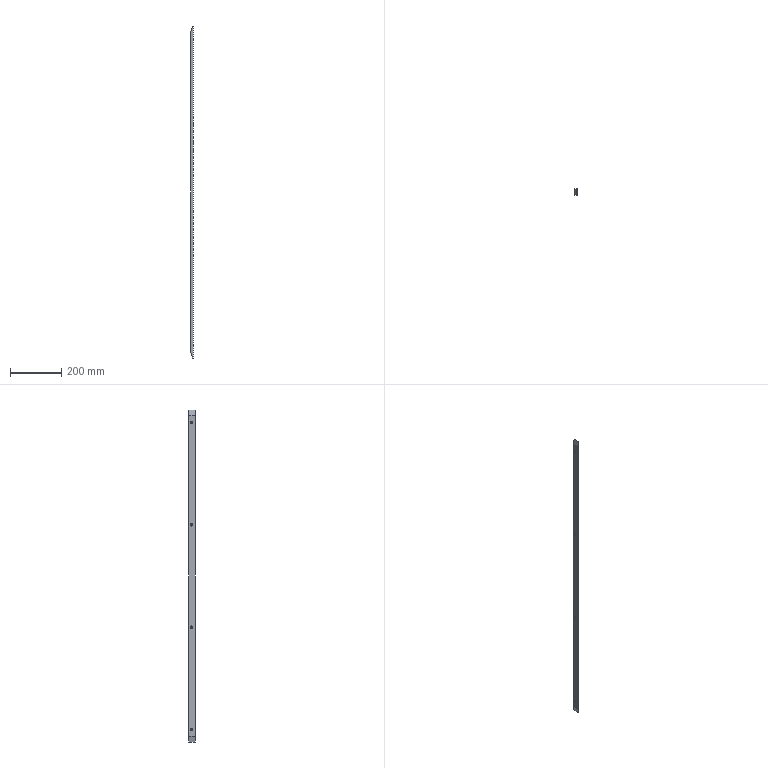Part | STEP file | 1 solid | 32 faces | box 8 x 25 x 1300 mm | volume 255560 mm3 | cylinder 16 | plane 8 | cone 8 | commonest cylinder face diameters 4.5 x8 9 x8